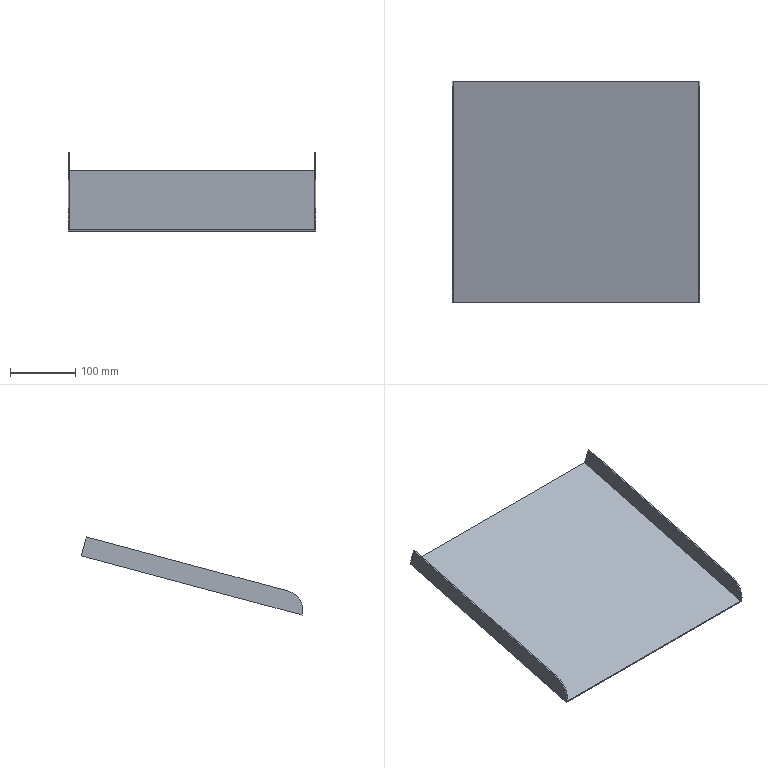Part | NX | features solid 2 | 1 solid | 12 faces | box 379.608 x 339.096 x 119.564 mm | volume 304153 mm3 | plane 10 | cylinder 2 | commonest cylinder face diameters 60 x2
STEP:
#1=CARTESIAN_POINT('',(-27.,-610.733,-523.089));
#2=VERTEX_POINT('',#1);
#3=CARTESIAN_POINT('',(-27.,-948.742,-613.658));
#4=VERTEX_POINT('',#3);
#5=CARTESIAN_POINT('',(-27.,-784.599,-569.676));
#6=DIRECTION('',(0.,-0.9659,-0.2588));
#7=VECTOR('',#6,1000.);
#8=LINE('',#5,#7);
#9=EDGE_CURVE('',#2,#4,#8,.T.);
#10=ORIENTED_EDGE('',*,*,#9,.F.);
#11=CARTESIAN_POINT('',(-402.608,-610.733,-523.089));
#12=VERTEX_POINT('',#11);
#13=CARTESIAN_POINT('',(-27.,-610.733,-523.089));
#14=DIRECTION('',(1.,0.,0.));
#15=VECTOR('',#14,1000.);
#16=LINE('',#13,#15);
#17=EDGE_CURVE('',#2,#12,#16,.F.);
#18=ORIENTED_EDGE('',*,*,#17,.T.);
#19=CARTESIAN_POINT('',(-402.608,-948.742,-613.658));
#20=VERTEX_POINT('',#19);
#21=CARTESIAN_POINT('',(-402.608,-766.757,-564.895));
#22=DIRECTION('',(0.,0.9659,0.2588));
#23=VECTOR('',#22,1000.);
#24=LINE('',#21,#23);
#25=EDGE_CURVE('',#12,#20,#24,.F.);
#26=ORIENTED_EDGE('',*,*,#25,.T.);
#27=CARTESIAN_POINT('',(-404.608,-948.742,-613.658));
#28=VERTEX_POINT('',#27);
#29=CARTESIAN_POINT('',(-250.794,-948.742,-613.658));
#30=DIRECTION('',(-1.,0.,0.));
#31=VECTOR('',#30,1000.);
#32=LINE('',#29,#31);
#33=EDGE_CURVE('',#28,#20,#32,.F.);
#34=ORIENTED_EDGE('',*,*,#33,.F.);
#35=CARTESIAN_POINT('',(-404.608,-948.807,-613.675));
#36=VERTEX_POINT('',#35);
#37=CARTESIAN_POINT('',(-404.608,-795.624,-572.63));
#38=DIRECTION('',(0.,0.9659,0.2588));
#39=VECTOR('',#38,1000.);
#40=LINE('',#37,#39);
#41=EDGE_CURVE('',#28,#36,#40,.F.);
#42=ORIENTED_EDGE('',*,*,#41,.T.);
#43=CARTESIAN_POINT('',(-25.,-948.807,-613.675));
#44=VERTEX_POINT('',#43);
#45=CARTESIAN_POINT('',(-27.,-948.807,-613.675));
#46=DIRECTION('',(1.,0.,0.));
#47=VECTOR('',#46,1000.);
#48=LINE('',#45,#47);
#49=EDGE_CURVE('',#44,#36,#48,.F.);
#50=ORIENTED_EDGE('',*,*,#49,.F.);
#51=CARTESIAN_POINT('',(-25.,-948.742,-613.658));
#52=VERTEX_POINT('',#51);
#53=CARTESIAN_POINT('',(-25.,-784.599,-569.676));
#54=DIRECTION('',(0.,-0.9659,-0.2588));
#55=VECTOR('',#54,1000.);
#56=LINE('',#53,#55);
#57=EDGE_CURVE('',#52,#44,#56,.T.);
#58=ORIENTED_EDGE('',*,*,#57,.F.);
#59=CARTESIAN_POINT('',(-15.,-948.742,-613.658));
#60=DIRECTION('',(1.,0.,0.));
#61=VECTOR('',#60,1000.);
#62=LINE('',#59,#61);
#63=EDGE_CURVE('',#4,#52,#62,.T.);
#64=ORIENTED_EDGE('',*,*,#63,.F.);
#65=EDGE_LOOP('',(#10,#18,#26,#34,#42,#50,#58,#64));
#66=FACE_BOUND('',#65,.T.);
#67=CARTESIAN_POINT('',(-27.,-784.599,-569.676));
#68=DIRECTION('',(0.,-0.2588,0.9659));
#69=DIRECTION('',(1.,0.,0.));
#70=AXIS2_PLACEMENT_3D('',#67,#68,#69);
#71=PLANE('',#70);
#72=ADVANCED_FACE('',(#66),#71,.T.);
#73=ORIENTED_EDGE('',*,*,#17,.F.);
#74=CARTESIAN_POINT('',(-27.,-617.98,-496.043));
#75=VERTEX_POINT('',#74);
#76=CARTESIAN_POINT('',(-27.,-610.215,-525.021));
#77=DIRECTION('',(0.,0.2588,-0.9659));
#78=VECTOR('',#77,1000.);
#79=LINE('',#76,#78);
#80=EDGE_CURVE('',#2,#75,#79,.F.);
#81=ORIENTED_EDGE('',*,*,#80,.T.);
#82=CARTESIAN_POINT('',(-25.,-617.98,-496.043));
#83=VERTEX_POINT('',#82);
#84=CARTESIAN_POINT('',(-27.,-617.98,-496.043));
#85=DIRECTION('',(-1.,0.,0.));
#86=VECTOR('',#85,1000.);
#87=LINE('',#84,#86);
#88=EDGE_CURVE('',#83,#75,#87,.T.);
#89=ORIENTED_EDGE('',*,*,#88,.F.);
#90=CARTESIAN_POINT('',(-25.,-610.215,-525.021));
#91=VERTEX_POINT('',#90);
#92=CARTESIAN_POINT('',(-25.,-610.215,-525.021));
#93=DIRECTION('',(0.,0.2588,-0.9659));
#94=VECTOR('',#93,1000.);
#95=LINE('',#92,#94);
#96=EDGE_CURVE('',#91,#83,#95,.F.);
#97=ORIENTED_EDGE('',*,*,#96,.F.);
#98=CARTESIAN_POINT('',(-404.608,-610.215,-525.021));
#99=VERTEX_POINT('',#98);
#100=CARTESIAN_POINT('',(-27.,-610.215,-525.021));
#101=DIRECTION('',(1.,0.,0.));
#102=VECTOR('',#101,1000.);
#103=LINE('',#100,#102);
#104=EDGE_CURVE('',#91,#99,#103,.F.);
#105=ORIENTED_EDGE('',*,*,#104,.T.);
#106=CARTESIAN_POINT('',(-404.608,-617.98,-496.043));
#107=VERTEX_POINT('',#106);
#108=CARTESIAN_POINT('',(-404.608,-610.215,-525.021));
#109=DIRECTION('',(0.,-0.2588,0.9659));
#110=VECTOR('',#109,1000.);
#111=LINE('',#108,#110);
#112=EDGE_CURVE('',#99,#107,#111,.T.);
#113=ORIENTED_EDGE('',*,*,#112,.T.);
#114=CARTESIAN_POINT('',(-402.608,-617.98,-496.043));
#115=VERTEX_POINT('',#114);
#116=CARTESIAN_POINT('',(-27.,-617.98,-496.043));
#117=DIRECTION('',(-1.,0.,0.));
#118=VECTOR('',#117,1000.);
#119=LINE('',#116,#118);
#120=EDGE_CURVE('',#107,#115,#119,.F.);
#121=ORIENTED_EDGE('',*,*,#120,.T.);
#122=CARTESIAN_POINT('',(-402.608,-610.215,-525.021));
#123=DIRECTION('',(0.,-0.2588,0.9659));
#124=VECTOR('',#123,1000.);
#125=LINE('',#122,#124);
#126=EDGE_CURVE('',#12,#115,#125,.T.);
#127=ORIENTED_EDGE('',*,*,#126,.F.);
#128=EDGE_LOOP('',(#73,#81,#89,#97,#105,#113,#121,#127));
#129=FACE_BOUND('',#128,.T.);
#130=CARTESIAN_POINT('',(-27.,-610.215,-525.021));
#131=DIRECTION('',(0.,0.9659,0.2588));
#132=DIRECTION('',(-1.,0.,0.));
#133=AXIS2_PLACEMENT_3D('',#130,#131,#132);
#134=PLANE('',#133);
#135=ADVANCED_FACE('',(#129),#134,.T.);
#136=CARTESIAN_POINT('',(-25.,-948.289,-615.607));
#137=VERTEX_POINT('',#136);
#138=CARTESIAN_POINT('',(-25.,-948.289,-615.607));
#139=DIRECTION('',(0.,-0.2588,0.9659));
#140=VECTOR('',#139,1000.);
#141=LINE('',#138,#140);
#142=EDGE_CURVE('',#137,#44,#141,.T.);
#143=ORIENTED_EDGE('',*,*,#142,.F.);
#144=CARTESIAN_POINT('',(-25.,-784.082,-571.608));
#145=DIRECTION('',(0.,-0.9659,-0.2588));
#146=VECTOR('',#145,1000.);
#147=LINE('',#144,#146);
#148=EDGE_CURVE('',#91,#137,#147,.T.);
#149=ORIENTED_EDGE('',*,*,#148,.F.);
#150=ORIENTED_EDGE('',*,*,#96,.T.);
#151=CARTESIAN_POINT('',(-25.,-927.076,-578.865));
#152=VERTEX_POINT('',#151);
#153=CARTESIAN_POINT('',(-25.,-791.846,-542.63));
#154=DIRECTION('',(0.,0.9659,0.2588));
#155=VECTOR('',#154,1000.);
#156=LINE('',#153,#155);
#157=EDGE_CURVE('',#83,#152,#156,.F.);
#158=ORIENTED_EDGE('',*,*,#157,.T.);
#159=CARTESIAN_POINT('',(-25.,-919.311,-607.843));
#160=DIRECTION('',(-1.,0.,0.));
#161=DIRECTION('',(0.,0.,1.));
#162=AXIS2_PLACEMENT_3D('',#159,#160,#161);
#163=CIRCLE('',#162,30.);
#164=EDGE_CURVE('',#152,#52,#163,.F.);
#165=ORIENTED_EDGE('',*,*,#164,.T.);
#166=ORIENTED_EDGE('',*,*,#57,.T.);
#167=EDGE_LOOP('',(#143,#149,#150,#158,#165,#166));
#168=FACE_BOUND('',#167,.T.);
#169=CARTESIAN_POINT('',(-25.,-784.082,-571.608));
#170=DIRECTION('',(-1.,0.,0.));
#171=DIRECTION('',(0.,-0.9659,-0.2588));
#172=AXIS2_PLACEMENT_3D('',#169,#170,#171);
#173=PLANE('',#172);
#174=ADVANCED_FACE('',(#168),#173,.F.);
#175=ORIENTED_EDGE('',*,*,#142,.T.);
#176=ORIENTED_EDGE('',*,*,#49,.T.);
#177=CARTESIAN_POINT('',(-404.608,-948.289,-615.607));
#178=VERTEX_POINT('',#177);
#179=CARTESIAN_POINT('',(-404.608,-936.311,-660.312));
#180=DIRECTION('',(0.,0.2588,-0.9659));
#181=VECTOR('',#180,1000.);
#182=LINE('',#179,#181);
#183=EDGE_CURVE('',#178,#36,#182,.F.);
#184=ORIENTED_EDGE('',*,*,#183,.F.);
#185=CARTESIAN_POINT('',(-27.,-948.289,-615.607));
#186=DIRECTION('',(-1.,0.,0.));
#187=VECTOR('',#186,1000.);
#188=LINE('',#185,#187);
#189=EDGE_CURVE('',#137,#178,#188,.T.);
#190=ORIENTED_EDGE('',*,*,#189,.F.);
#191=EDGE_LOOP('',(#175,#176,#184,#190));
#192=FACE_BOUND('',#191,.T.);
#193=CARTESIAN_POINT('',(-27.,-948.289,-615.607));
#194=DIRECTION('',(0.,0.9659,0.2588));
#195=DIRECTION('',(-1.,0.,0.));
#196=AXIS2_PLACEMENT_3D('',#193,#194,#195);
#197=PLANE('',#196);
#198=ADVANCED_FACE('',(#192),#197,.F.);
#199=ORIENTED_EDGE('',*,*,#41,.F.);
#200=CARTESIAN_POINT('',(-404.608,-927.076,-578.865));
#201=VERTEX_POINT('',#200);
#202=CARTESIAN_POINT('',(-404.608,-919.311,-607.843));
#203=DIRECTION('',(-1.,0.,0.));
#204=DIRECTION('',(0.,0.,1.));
#205=AXIS2_PLACEMENT_3D('',#202,#203,#204);
#206=CIRCLE('',#205,30.);
#207=EDGE_CURVE('',#28,#201,#206,.T.);
#208=ORIENTED_EDGE('',*,*,#207,.T.);
#209=CARTESIAN_POINT('',(-404.608,-791.846,-542.63));
#210=DIRECTION('',(0.,0.9659,0.2588));
#211=VECTOR('',#210,1000.);
#212=LINE('',#209,#211);
#213=EDGE_CURVE('',#107,#201,#212,.F.);
#214=ORIENTED_EDGE('',*,*,#213,.F.);
#215=ORIENTED_EDGE('',*,*,#112,.F.);
#216=CARTESIAN_POINT('',(-404.608,-795.107,-574.562));
#217=DIRECTION('',(0.,0.9659,0.2588));
#218=VECTOR('',#217,1000.);
#219=LINE('',#216,#218);
#220=EDGE_CURVE('',#99,#178,#219,.F.);
#221=ORIENTED_EDGE('',*,*,#220,.T.);
#222=ORIENTED_EDGE('',*,*,#183,.T.);
#223=EDGE_LOOP('',(#199,#208,#214,#215,#221,#222));
#224=FACE_BOUND('',#223,.T.);
#225=CARTESIAN_POINT('',(-404.608,-783.128,-619.267));
#226=DIRECTION('',(-1.,0.,0.));
#227=DIRECTION('',(0.,-0.9397,-0.342));
#228=AXIS2_PLACEMENT_3D('',#225,#226,#227);
#229=PLANE('',#228);
#230=ADVANCED_FACE('',(#224),#229,.T.);
#231=ORIENTED_EDGE('',*,*,#220,.F.);
#232=ORIENTED_EDGE('',*,*,#104,.F.);
#233=ORIENTED_EDGE('',*,*,#148,.T.);
#234=ORIENTED_EDGE('',*,*,#189,.T.);
#235=EDGE_LOOP('',(#231,#232,#233,#234));
#236=FACE_BOUND('',#235,.T.);
#237=CARTESIAN_POINT('',(-27.,-784.082,-571.608));
#238=DIRECTION('',(0.,-0.2588,0.9659));
#239=DIRECTION('',(1.,0.,0.));
#240=AXIS2_PLACEMENT_3D('',#237,#238,#239);
#241=PLANE('',#240);
#242=ADVANCED_FACE('',(#236),#241,.F.);
#243=ORIENTED_EDGE('',*,*,#213,.T.);
#244=CARTESIAN_POINT('',(-402.608,-927.076,-578.865));
#245=VERTEX_POINT('',#244);
#246=CARTESIAN_POINT('',(-250.794,-927.076,-578.865));
#247=DIRECTION('',(-1.,0.,0.));
#248=VECTOR('',#247,1000.);
#249=LINE('',#246,#248);
#250=EDGE_CURVE('',#201,#245,#249,.F.);
#251=ORIENTED_EDGE('',*,*,#250,.T.);
#252=CARTESIAN_POINT('',(-402.608,-791.846,-542.63));
#253=DIRECTION('',(0.,0.9659,0.2588));
#254=VECTOR('',#253,1000.);
#255=LINE('',#252,#254);
#256=EDGE_CURVE('',#115,#245,#255,.F.);
#257=ORIENTED_EDGE('',*,*,#256,.F.);
#258=ORIENTED_EDGE('',*,*,#120,.F.);
#259=EDGE_LOOP('',(#243,#251,#257,#258));
#260=FACE_BOUND('',#259,.T.);
#261=CARTESIAN_POINT('',(-250.794,-791.846,-542.63));
#262=DIRECTION('',(0.,0.2588,-0.9659));
#263=DIRECTION('',(0.,-0.9659,-0.2588));
#264=AXIS2_PLACEMENT_3D('',#261,#262,#263);
#265=PLANE('',#264);
#266=ADVANCED_FACE('',(#260),#265,.F.);
#267=ORIENTED_EDGE('',*,*,#25,.F.);
#268=ORIENTED_EDGE('',*,*,#126,.T.);
#269=ORIENTED_EDGE('',*,*,#256,.T.);
#270=CARTESIAN_POINT('',(-402.608,-919.311,-607.843));
#271=DIRECTION('',(-1.,0.,0.));
#272=DIRECTION('',(0.,0.,1.));
#273=AXIS2_PLACEMENT_3D('',#270,#271,#272);
#274=CIRCLE('',#273,30.);
#275=EDGE_CURVE('',#245,#20,#274,.F.);
#276=ORIENTED_EDGE('',*,*,#275,.T.);
#277=EDGE_LOOP('',(#267,#268,#269,#276));
#278=FACE_BOUND('',#277,.T.);
#279=CARTESIAN_POINT('',(-402.608,-754.937,-609.006));
#280=DIRECTION('',(-1.,0.,0.));
#281=DIRECTION('',(0.,0.,1.));
#282=AXIS2_PLACEMENT_3D('',#279,#280,#281);
#283=PLANE('',#282);
#284=ADVANCED_FACE('',(#278),#283,.F.);
#285=ORIENTED_EDGE('',*,*,#207,.F.);
#286=ORIENTED_EDGE('',*,*,#33,.T.);
#287=ORIENTED_EDGE('',*,*,#275,.F.);
#288=ORIENTED_EDGE('',*,*,#250,.F.);
#289=EDGE_LOOP('',(#285,#286,#287,#288));
#290=FACE_BOUND('',#289,.T.);
#291=CARTESIAN_POINT('',(-250.794,-919.311,-607.843));
#292=DIRECTION('',(-1.,0.,0.));
#293=DIRECTION('',(0.,-0.2588,0.9659));
#294=AXIS2_PLACEMENT_3D('',#291,#292,#293);
#295=CYLINDRICAL_SURFACE('',#294,30.);
#296=ADVANCED_FACE('',(#290),#295,.T.);
#297=CARTESIAN_POINT('',(-27.,-927.076,-578.865));
#298=VERTEX_POINT('',#297);
#299=CARTESIAN_POINT('',(-27.,-791.846,-542.63));
#300=DIRECTION('',(0.,0.9659,0.2588));
#301=VECTOR('',#300,1000.);
#302=LINE('',#299,#301);
#303=EDGE_CURVE('',#75,#298,#302,.F.);
#304=ORIENTED_EDGE('',*,*,#303,.T.);
#305=CARTESIAN_POINT('',(-15.,-927.076,-578.865));
#306=DIRECTION('',(-1.,0.,0.));
#307=VECTOR('',#306,1000.);
#308=LINE('',#305,#307);
#309=EDGE_CURVE('',#298,#152,#308,.F.);
#310=ORIENTED_EDGE('',*,*,#309,.T.);
#311=ORIENTED_EDGE('',*,*,#157,.F.);
#312=ORIENTED_EDGE('',*,*,#88,.T.);
#313=EDGE_LOOP('',(#304,#310,#311,#312));
#314=FACE_BOUND('',#313,.T.);
#315=CARTESIAN_POINT('',(-15.,-791.846,-542.63));
#316=DIRECTION('',(0.,0.2588,-0.9659));
#317=DIRECTION('',(0.,-0.9659,-0.2588));
#318=AXIS2_PLACEMENT_3D('',#315,#316,#317);
#319=PLANE('',#318);
#320=ADVANCED_FACE('',(#314),#319,.F.);
#321=ORIENTED_EDGE('',*,*,#80,.F.);
#322=ORIENTED_EDGE('',*,*,#9,.T.);
#323=CARTESIAN_POINT('',(-27.,-919.311,-607.843));
#324=DIRECTION('',(-1.,0.,0.));
#325=DIRECTION('',(0.,0.,1.));
#326=AXIS2_PLACEMENT_3D('',#323,#324,#325);
#327=CIRCLE('',#326,30.);
#328=EDGE_CURVE('',#4,#298,#327,.T.);
#329=ORIENTED_EDGE('',*,*,#328,.T.);
#330=ORIENTED_EDGE('',*,*,#303,.F.);
#331=EDGE_LOOP('',(#321,#322,#329,#330));
#332=FACE_BOUND('',#331,.T.);
#333=CARTESIAN_POINT('',(-27.,-784.082,-571.608));
#334=DIRECTION('',(-1.,0.,0.));
#335=DIRECTION('',(0.,-0.2588,0.9659));
#336=AXIS2_PLACEMENT_3D('',#333,#334,#335);
#337=PLANE('',#336);
#338=ADVANCED_FACE('',(#332),#337,.T.);
#339=ORIENTED_EDGE('',*,*,#328,.F.);
#340=ORIENTED_EDGE('',*,*,#63,.T.);
#341=ORIENTED_EDGE('',*,*,#164,.F.);
#342=ORIENTED_EDGE('',*,*,#309,.F.);
#343=EDGE_LOOP('',(#339,#340,#341,#342));
#344=FACE_BOUND('',#343,.T.);
#345=CARTESIAN_POINT('',(-15.,-919.311,-607.843));
#346=DIRECTION('',(1.,0.,0.));
#347=DIRECTION('',(0.,0.2588,-0.9659));
#348=AXIS2_PLACEMENT_3D('',#345,#346,#347);
#349=CYLINDRICAL_SURFACE('',#348,30.);
#350=ADVANCED_FACE('',(#344),#349,.T.);
#351=CLOSED_SHELL('',(#72,#135,#174,#198,#230,#242,#266,#284,#296,#320,#338,#350));
#352=MANIFOLD_SOLID_BREP('',#351);
#353=(LENGTH_UNIT()NAMED_UNIT(*)SI_UNIT(.MILLI.,.METRE.));
#354=UNCERTAINTY_MEASURE_WITH_UNIT(LENGTH_MEASURE(0.00001),#353,'','');
#355=(NAMED_UNIT(*)PLANE_ANGLE_UNIT()SI_UNIT($,.RADIAN.));
#356=(NAMED_UNIT(*)SI_UNIT($,.STERADIAN.)SOLID_ANGLE_UNIT());
#357=(GEOMETRIC_REPRESENTATION_CONTEXT(3)GLOBAL_UNCERTAINTY_ASSIGNED_CONTEXT((#354))GLOBAL_UNIT_ASSIGNED_CONTEXT((#353,#355,#356))REPRESENTATION_CONTEXT('',''));
#358=ADVANCED_BREP_SHAPE_REPRESENTATION('',(#352),#357);